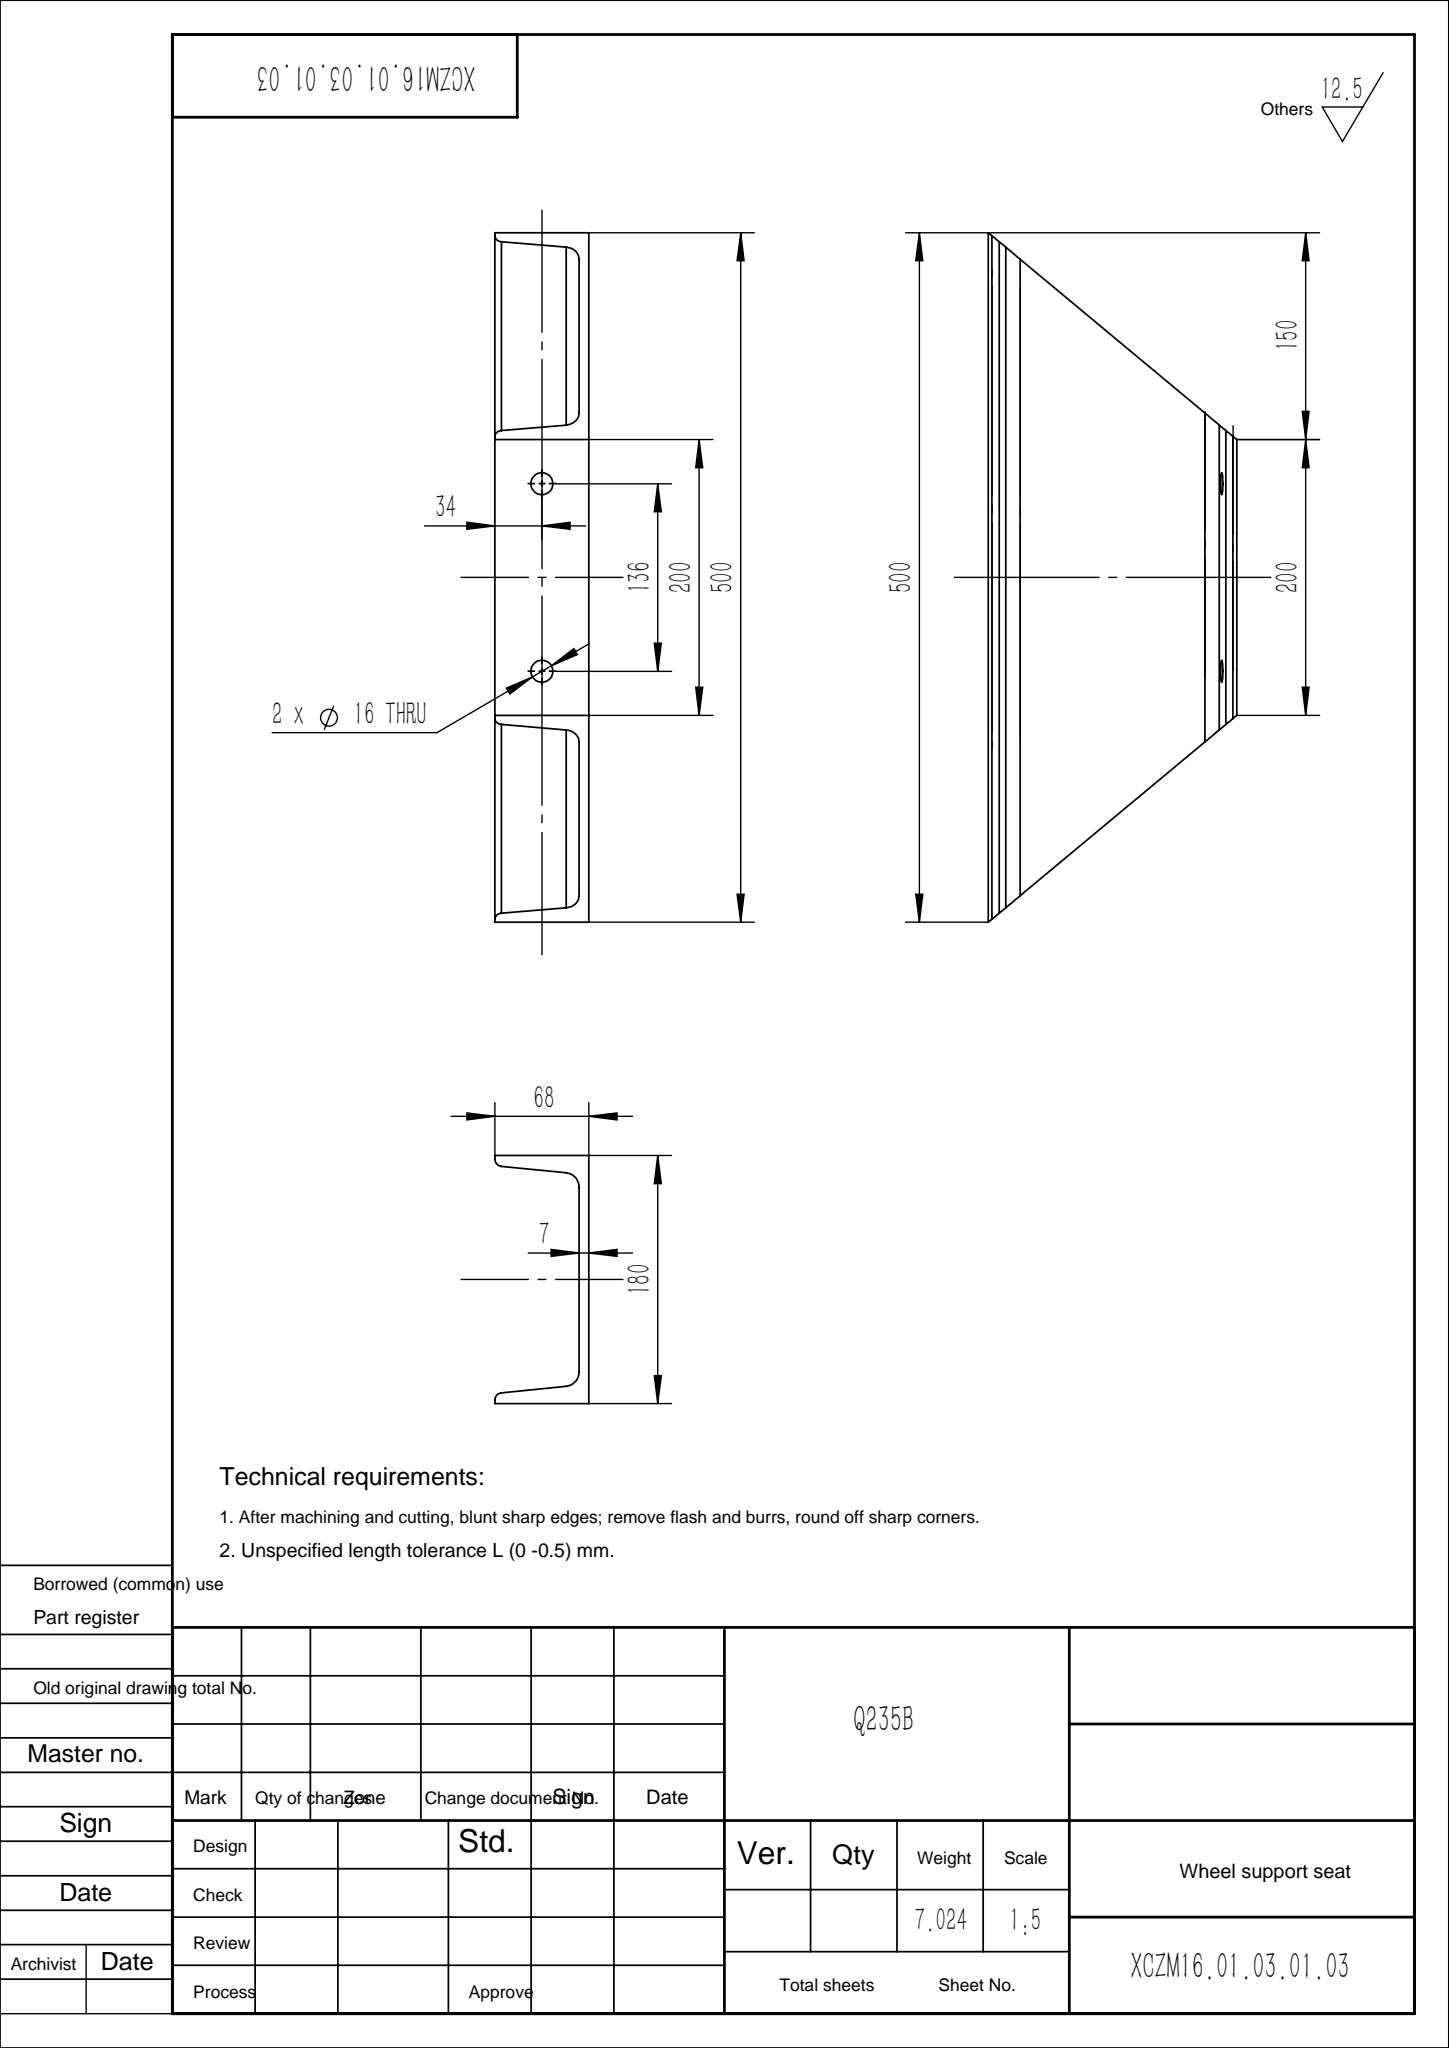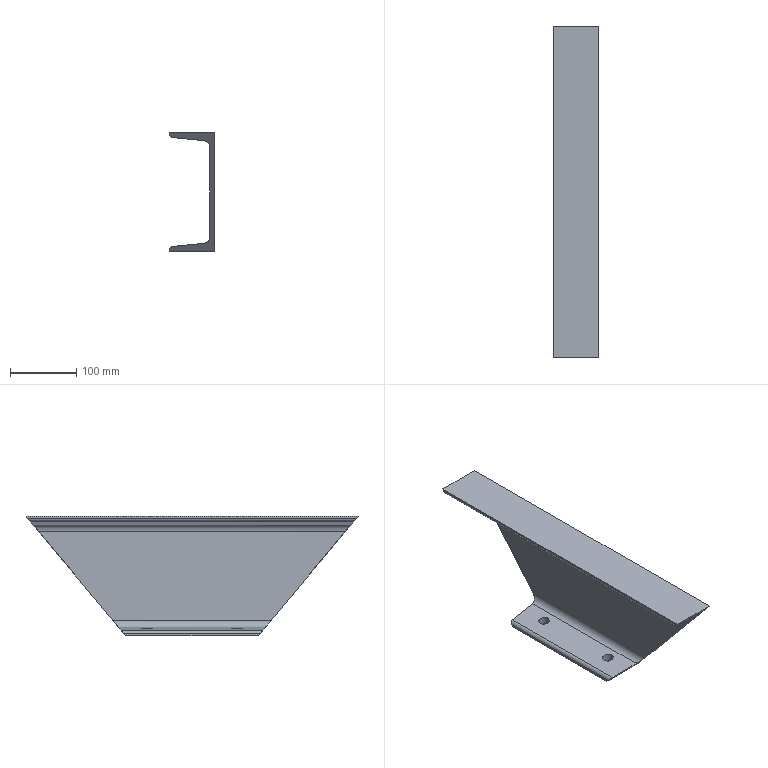Part | SolidWorks | features HoleWzd 1, ICE 1, WeldMemberFeat 1, WeldmentFeature 1 | 1 solid | 18 faces | box 68 x 500 x 180 mm | volume 894795 mm3 | plane 10 | cylinder 8 | commonest cylinder face diameters 16 x4 10.5 x2 21 x2
STEP:
#1=CARTESIAN_POINT('',(-26.,318.,11.65));
#2=VERTEX_POINT('',#1);
#3=CARTESIAN_POINT('',(-42.,318.,10.05));
#4=VERTEX_POINT('',#3);
#5=CARTESIAN_POINT('',(-26.,318.,11.65));
#6=CARTESIAN_POINT('',(-26.,302.,11.65));
#7=CARTESIAN_POINT('',(-42.,302.,10.05));
#8=CARTESIAN_POINT('',(-42.,318.,10.05));
#9=(BOUNDED_CURVE()B_SPLINE_CURVE(3,(#5,#6,#7,#8),.UNSPECIFIED.,.F.,.F.)B_SPLINE_CURVE_WITH_KNOTS((4,4),(3.142,6.283),.UNSPECIFIED.)CURVE()GEOMETRIC_REPRESENTATION_ITEM()RATIONAL_B_SPLINE_CURVE((1.,0.3333,0.3333,1.))REPRESENTATION_ITEM(''));
#10=EDGE_CURVE('',#2,#4,#9,.T.);
#11=ORIENTED_EDGE('',*,*,#10,.F.);
#12=CARTESIAN_POINT('',(-26.,318.,0.));
#13=VERTEX_POINT('',#12);
#14=CARTESIAN_POINT('',(-26.,318.,0.));
#15=DIRECTION('',(0.,0.,-1.));
#16=VECTOR('',#15,1000.);
#17=LINE('',#14,#16);
#18=EDGE_CURVE('',#2,#13,#17,.T.);
#19=ORIENTED_EDGE('',*,*,#18,.T.);
#20=CARTESIAN_POINT('',(-42.,318.,0.));
#21=VERTEX_POINT('',#20);
#22=CARTESIAN_POINT('',(-34.,318.,0.));
#23=DIRECTION('',(0.,0.,-1.));
#24=DIRECTION('',(-1.,0.,0.));
#25=AXIS2_PLACEMENT_3D('',#22,#23,#24);
#26=CIRCLE('',#25,8.);
#27=EDGE_CURVE('',#13,#21,#26,.T.);
#28=ORIENTED_EDGE('',*,*,#27,.T.);
#29=CARTESIAN_POINT('',(-42.,318.,0.));
#30=DIRECTION('',(0.,0.,-1.));
#31=VECTOR('',#30,1000.);
#32=LINE('',#29,#31);
#33=EDGE_CURVE('',#4,#21,#32,.T.);
#34=ORIENTED_EDGE('',*,*,#33,.F.);
#35=EDGE_LOOP('',(#11,#19,#28,#34));
#36=FACE_OUTER_BOUND('',#35,.T.);
#37=CARTESIAN_POINT('',(-34.,318.,0.));
#38=DIRECTION('',(0.,0.,-1.));
#39=DIRECTION('',(-1.,0.,0.));
#40=AXIS2_PLACEMENT_3D('',#37,#38,#39);
#41=CYLINDRICAL_SURFACE('',#40,8.);
#42=ADVANCED_FACE('',(#36),#41,.F.);
#43=CARTESIAN_POINT('',(-26.,182.,11.65));
#44=VERTEX_POINT('',#43);
#45=CARTESIAN_POINT('',(-42.,182.,10.05));
#46=VERTEX_POINT('',#45);
#47=CARTESIAN_POINT('',(-26.,182.,11.65));
#48=CARTESIAN_POINT('',(-26.,166.,11.65));
#49=CARTESIAN_POINT('',(-42.,166.,10.05));
#50=CARTESIAN_POINT('',(-42.,182.,10.05));
#51=(BOUNDED_CURVE()B_SPLINE_CURVE(3,(#47,#48,#49,#50),.UNSPECIFIED.,.F.,.F.)B_SPLINE_CURVE_WITH_KNOTS((4,4),(3.142,6.283),.UNSPECIFIED.)CURVE()GEOMETRIC_REPRESENTATION_ITEM()RATIONAL_B_SPLINE_CURVE((1.,0.3333,0.3333,1.))REPRESENTATION_ITEM(''));
#52=EDGE_CURVE('',#44,#46,#51,.T.);
#53=ORIENTED_EDGE('',*,*,#52,.F.);
#54=CARTESIAN_POINT('',(-26.,182.,0.));
#55=VERTEX_POINT('',#54);
#56=CARTESIAN_POINT('',(-26.,182.,0.));
#57=DIRECTION('',(0.,0.,-1.));
#58=VECTOR('',#57,1000.);
#59=LINE('',#56,#58);
#60=EDGE_CURVE('',#44,#55,#59,.T.);
#61=ORIENTED_EDGE('',*,*,#60,.T.);
#62=CARTESIAN_POINT('',(-42.,182.,0.));
#63=VERTEX_POINT('',#62);
#64=CARTESIAN_POINT('',(-34.,182.,0.));
#65=DIRECTION('',(0.,0.,-1.));
#66=DIRECTION('',(-1.,0.,0.));
#67=AXIS2_PLACEMENT_3D('',#64,#65,#66);
#68=CIRCLE('',#67,8.);
#69=EDGE_CURVE('',#55,#63,#68,.T.);
#70=ORIENTED_EDGE('',*,*,#69,.T.);
#71=CARTESIAN_POINT('',(-42.,182.,0.));
#72=DIRECTION('',(0.,0.,-1.));
#73=VECTOR('',#72,1000.);
#74=LINE('',#71,#73);
#75=EDGE_CURVE('',#46,#63,#74,.T.);
#76=ORIENTED_EDGE('',*,*,#75,.F.);
#77=EDGE_LOOP('',(#53,#61,#70,#76));
#78=FACE_OUTER_BOUND('',#77,.T.);
#79=CARTESIAN_POINT('',(-34.,182.,0.));
#80=DIRECTION('',(0.,0.,-1.));
#81=DIRECTION('',(-1.,0.,0.));
#82=AXIS2_PLACEMENT_3D('',#79,#80,#81);
#83=CYLINDRICAL_SURFACE('',#82,8.);
#84=ADVANCED_FACE('',(#78),#83,.F.);
#85=CARTESIAN_POINT('',(-63.272,493.398,172.077));
#86=VERTEX_POINT('',#85);
#87=CARTESIAN_POINT('',(-68.,497.751,177.301));
#88=VERTEX_POINT('',#87);
#89=CARTESIAN_POINT('',(-63.272,493.398,172.077));
#90=CARTESIAN_POINT('',(-66.096,493.633,172.36));
#91=CARTESIAN_POINT('',(-68.,495.386,174.464));
#92=CARTESIAN_POINT('',(-68.,497.751,177.301));
#93=(BOUNDED_CURVE()B_SPLINE_CURVE(3,(#89,#90,#91,#92),.UNSPECIFIED.,.F.,.F.)B_SPLINE_CURVE_WITH_KNOTS((4,4),(0.09967,1.571),.UNSPECIFIED.)CURVE()GEOMETRIC_REPRESENTATION_ITEM()RATIONAL_B_SPLINE_CURVE((1.,0.8276,0.8276,1.))REPRESENTATION_ITEM(''));
#94=EDGE_CURVE('',#86,#88,#93,.T.);
#95=ORIENTED_EDGE('',*,*,#94,.F.);
#96=CARTESIAN_POINT('',(-63.272,6.602,172.077));
#97=VERTEX_POINT('',#96);
#98=CARTESIAN_POINT('',(-63.272,500.,172.077));
#99=DIRECTION('',(0.,-1.,0.));
#100=VECTOR('',#99,1000.);
#101=LINE('',#98,#100);
#102=EDGE_CURVE('',#86,#97,#101,.T.);
#103=ORIENTED_EDGE('',*,*,#102,.T.);
#104=CARTESIAN_POINT('',(-68.,2.249,177.301));
#105=VERTEX_POINT('',#104);
#106=CARTESIAN_POINT('',(-68.,2.249,177.301));
#107=CARTESIAN_POINT('',(-68.,4.614,174.464));
#108=CARTESIAN_POINT('',(-66.096,6.367,172.36));
#109=CARTESIAN_POINT('',(-63.272,6.602,172.077));
#110=(BOUNDED_CURVE()B_SPLINE_CURVE(3,(#106,#107,#108,#109),.UNSPECIFIED.,.F.,.F.)B_SPLINE_CURVE_WITH_KNOTS((4,4),(1.571,3.042),.UNSPECIFIED.)CURVE()GEOMETRIC_REPRESENTATION_ITEM()RATIONAL_B_SPLINE_CURVE((1.,0.8276,0.8276,1.))REPRESENTATION_ITEM(''));
#111=EDGE_CURVE('',#105,#97,#110,.T.);
#112=ORIENTED_EDGE('',*,*,#111,.F.);
#113=CARTESIAN_POINT('',(-68.,500.,177.301));
#114=DIRECTION('',(0.,-1.,0.));
#115=VECTOR('',#114,1000.);
#116=LINE('',#113,#115);
#117=EDGE_CURVE('',#88,#105,#116,.T.);
#118=ORIENTED_EDGE('',*,*,#117,.F.);
#119=EDGE_LOOP('',(#95,#103,#112,#118));
#120=FACE_OUTER_BOUND('',#119,.T.);
#121=CARTESIAN_POINT('',(-62.75,500.,177.301));
#122=DIRECTION('',(0.,-1.,0.));
#123=DIRECTION('',(0.,0.,-1.));
#124=AXIS2_PLACEMENT_3D('',#121,#122,#123);
#125=CYLINDRICAL_SURFACE('',#124,5.25);
#126=ADVANCED_FACE('',(#120),#125,.T.);
#127=CARTESIAN_POINT('',(-68.,500.,180.));
#128=VERTEX_POINT('',#127);
#129=CARTESIAN_POINT('',(-68.,500.,180.));
#130=DIRECTION('',(0.,0.6402,0.7682));
#131=VECTOR('',#130,1000.);
#132=LINE('',#129,#131);
#133=EDGE_CURVE('',#88,#128,#132,.T.);
#134=ORIENTED_EDGE('',*,*,#133,.F.);
#135=ORIENTED_EDGE('',*,*,#117,.T.);
#136=CARTESIAN_POINT('',(-68.,0.,180.));
#137=VERTEX_POINT('',#136);
#138=CARTESIAN_POINT('',(-68.,0.,180.));
#139=DIRECTION('',(0.,0.6402,-0.7682));
#140=VECTOR('',#139,1000.);
#141=LINE('',#138,#140);
#142=EDGE_CURVE('',#137,#105,#141,.T.);
#143=ORIENTED_EDGE('',*,*,#142,.F.);
#144=CARTESIAN_POINT('',(-68.,500.,180.));
#145=DIRECTION('',(0.,-1.,0.));
#146=VECTOR('',#145,1000.);
#147=LINE('',#144,#146);
#148=EDGE_CURVE('',#128,#137,#147,.T.);
#149=ORIENTED_EDGE('',*,*,#148,.F.);
#150=EDGE_LOOP('',(#134,#135,#143,#149));
#151=FACE_OUTER_BOUND('',#150,.T.);
#152=CARTESIAN_POINT('',(-68.,500.,180.));
#153=DIRECTION('',(1.,0.,0.));
#154=DIRECTION('',(0.,0.,-1.));
#155=AXIS2_PLACEMENT_3D('',#152,#153,#154);
#156=PLANE('',#155);
#157=ADVANCED_FACE('',(#151),#156,.F.);
#158=CARTESIAN_POINT('',(0.,350.,0.));
#159=VERTEX_POINT('',#158);
#160=CARTESIAN_POINT('',(0.,500.,180.));
#161=VERTEX_POINT('',#160);
#162=CARTESIAN_POINT('',(0.,500.,180.));
#163=DIRECTION('',(0.,0.6402,0.7682));
#164=VECTOR('',#163,1000.);
#165=LINE('',#162,#164);
#166=EDGE_CURVE('',#159,#161,#165,.T.);
#167=ORIENTED_EDGE('',*,*,#166,.T.);
#168=CARTESIAN_POINT('',(0.,0.,180.));
#169=VERTEX_POINT('',#168);
#170=CARTESIAN_POINT('',(0.,500.,180.));
#171=DIRECTION('',(0.,-1.,0.));
#172=VECTOR('',#171,1000.);
#173=LINE('',#170,#172);
#174=EDGE_CURVE('',#161,#169,#173,.T.);
#175=ORIENTED_EDGE('',*,*,#174,.T.);
#176=CARTESIAN_POINT('',(0.,150.,0.));
#177=VERTEX_POINT('',#176);
#178=CARTESIAN_POINT('',(0.,0.,180.));
#179=DIRECTION('',(0.,0.6402,-0.7682));
#180=VECTOR('',#179,1000.);
#181=LINE('',#178,#180);
#182=EDGE_CURVE('',#169,#177,#181,.T.);
#183=ORIENTED_EDGE('',*,*,#182,.T.);
#184=CARTESIAN_POINT('',(0.,500.,0.));
#185=DIRECTION('',(0.,-1.,0.));
#186=VECTOR('',#185,1000.);
#187=LINE('',#184,#186);
#188=EDGE_CURVE('',#159,#177,#187,.T.);
#189=ORIENTED_EDGE('',*,*,#188,.F.);
#190=EDGE_LOOP('',(#167,#175,#183,#189));
#191=FACE_OUTER_BOUND('',#190,.T.);
#192=CARTESIAN_POINT('',(0.,500.,180.));
#193=DIRECTION('',(-1.,0.,0.));
#194=DIRECTION('',(0.,0.,1.));
#195=AXIS2_PLACEMENT_3D('',#192,#193,#194);
#196=PLANE('',#195);
#197=ADVANCED_FACE('',(#191),#196,.F.);
#198=CARTESIAN_POINT('',(-34.,318.,0.));
#199=DIRECTION('',(0.,0.,-1.));
#200=DIRECTION('',(-1.,0.,0.));
#201=AXIS2_PLACEMENT_3D('',#198,#199,#200);
#202=CIRCLE('',#201,8.);
#203=EDGE_CURVE('',#21,#13,#202,.T.);
#204=ORIENTED_EDGE('',*,*,#203,.F.);
#205=ORIENTED_EDGE('',*,*,#27,.F.);
#206=EDGE_LOOP('',(#204,#205));
#207=FACE_BOUND('',#206,.T.);
#208=CARTESIAN_POINT('',(-34.,182.,0.));
#209=DIRECTION('',(0.,0.,-1.));
#210=DIRECTION('',(-1.,0.,0.));
#211=AXIS2_PLACEMENT_3D('',#208,#209,#210);
#212=CIRCLE('',#211,8.);
#213=EDGE_CURVE('',#63,#55,#212,.T.);
#214=ORIENTED_EDGE('',*,*,#213,.F.);
#215=ORIENTED_EDGE('',*,*,#69,.F.);
#216=EDGE_LOOP('',(#214,#215));
#217=FACE_BOUND('',#216,.T.);
#218=CARTESIAN_POINT('',(-68.,350.,0.));
#219=VERTEX_POINT('',#218);
#220=CARTESIAN_POINT('',(-68.,350.,0.));
#221=DIRECTION('',(1.,0.,0.));
#222=VECTOR('',#221,1000.);
#223=LINE('',#220,#222);
#224=EDGE_CURVE('',#219,#159,#223,.T.);
#225=ORIENTED_EDGE('',*,*,#224,.T.);
#226=ORIENTED_EDGE('',*,*,#188,.T.);
#227=CARTESIAN_POINT('',(-68.,150.,0.));
#228=VERTEX_POINT('',#227);
#229=CARTESIAN_POINT('',(-68.,150.,0.));
#230=DIRECTION('',(1.,0.,0.));
#231=VECTOR('',#230,1000.);
#232=LINE('',#229,#231);
#233=EDGE_CURVE('',#228,#177,#232,.T.);
#234=ORIENTED_EDGE('',*,*,#233,.F.);
#235=CARTESIAN_POINT('',(-68.,500.,0.));
#236=DIRECTION('',(0.,-1.,0.));
#237=VECTOR('',#236,1000.);
#238=LINE('',#235,#237);
#239=EDGE_CURVE('',#219,#228,#238,.T.);
#240=ORIENTED_EDGE('',*,*,#239,.F.);
#241=EDGE_LOOP('',(#225,#226,#234,#240));
#242=FACE_OUTER_BOUND('',#241,.T.);
#243=CARTESIAN_POINT('',(-68.,500.,0.));
#244=DIRECTION('',(0.,0.,1.));
#245=DIRECTION('',(1.,0.,0.));
#246=AXIS2_PLACEMENT_3D('',#243,#244,#245);
#247=PLANE('',#246);
#248=ADVANCED_FACE('',(#207,#217,#242),#247,.F.);
#249=CARTESIAN_POINT('',(-68.,352.249,2.699));
#250=VERTEX_POINT('',#249);
#251=CARTESIAN_POINT('',(-68.,500.,180.));
#252=DIRECTION('',(0.,0.6402,0.7682));
#253=VECTOR('',#252,1000.);
#254=LINE('',#251,#253);
#255=EDGE_CURVE('',#219,#250,#254,.T.);
#256=ORIENTED_EDGE('',*,*,#255,.F.);
#257=ORIENTED_EDGE('',*,*,#239,.T.);
#258=CARTESIAN_POINT('',(-68.,147.751,2.699));
#259=VERTEX_POINT('',#258);
#260=CARTESIAN_POINT('',(-68.,0.,180.));
#261=DIRECTION('',(0.,0.6402,-0.7682));
#262=VECTOR('',#261,1000.);
#263=LINE('',#260,#262);
#264=EDGE_CURVE('',#259,#228,#263,.T.);
#265=ORIENTED_EDGE('',*,*,#264,.F.);
#266=CARTESIAN_POINT('',(-68.,500.,2.699));
#267=DIRECTION('',(0.,-1.,0.));
#268=VECTOR('',#267,1000.);
#269=LINE('',#266,#268);
#270=EDGE_CURVE('',#250,#259,#269,.T.);
#271=ORIENTED_EDGE('',*,*,#270,.F.);
#272=EDGE_LOOP('',(#256,#257,#265,#271));
#273=FACE_OUTER_BOUND('',#272,.T.);
#274=CARTESIAN_POINT('',(-68.,500.,0.));
#275=DIRECTION('',(1.,0.,0.));
#276=DIRECTION('',(0.,0.,-1.));
#277=AXIS2_PLACEMENT_3D('',#274,#275,#276);
#278=PLANE('',#277);
#279=ADVANCED_FACE('',(#273),#278,.F.);
#280=CARTESIAN_POINT('',(-63.272,356.602,7.923));
#281=VERTEX_POINT('',#280);
#282=CARTESIAN_POINT('',(-68.,352.249,2.699));
#283=CARTESIAN_POINT('',(-68.,354.614,5.536));
#284=CARTESIAN_POINT('',(-66.096,356.367,7.64));
#285=CARTESIAN_POINT('',(-63.272,356.602,7.923));
#286=(BOUNDED_CURVE()B_SPLINE_CURVE(3,(#282,#283,#284,#285),.UNSPECIFIED.,.F.,.F.)B_SPLINE_CURVE_WITH_KNOTS((4,4),(1.571,3.042),.UNSPECIFIED.)CURVE()GEOMETRIC_REPRESENTATION_ITEM()RATIONAL_B_SPLINE_CURVE((1.,0.8276,0.8276,1.))REPRESENTATION_ITEM(''));
#287=EDGE_CURVE('',#250,#281,#286,.T.);
#288=ORIENTED_EDGE('',*,*,#287,.F.);
#289=ORIENTED_EDGE('',*,*,#270,.T.);
#290=CARTESIAN_POINT('',(-63.272,143.398,7.923));
#291=VERTEX_POINT('',#290);
#292=CARTESIAN_POINT('',(-63.272,143.398,7.923));
#293=CARTESIAN_POINT('',(-66.096,143.633,7.64));
#294=CARTESIAN_POINT('',(-68.,145.386,5.536));
#295=CARTESIAN_POINT('',(-68.,147.751,2.699));
#296=(BOUNDED_CURVE()B_SPLINE_CURVE(3,(#292,#293,#294,#295),.UNSPECIFIED.,.F.,.F.)B_SPLINE_CURVE_WITH_KNOTS((4,4),(0.09967,1.571),.UNSPECIFIED.)CURVE()GEOMETRIC_REPRESENTATION_ITEM()RATIONAL_B_SPLINE_CURVE((1.,0.8276,0.8276,1.))REPRESENTATION_ITEM(''));
#297=EDGE_CURVE('',#291,#259,#296,.T.);
#298=ORIENTED_EDGE('',*,*,#297,.F.);
#299=CARTESIAN_POINT('',(-63.272,500.,7.923));
#300=DIRECTION('',(0.,-1.,0.));
#301=VECTOR('',#300,1000.);
#302=LINE('',#299,#301);
#303=EDGE_CURVE('',#281,#291,#302,.T.);
#304=ORIENTED_EDGE('',*,*,#303,.F.);
#305=EDGE_LOOP('',(#288,#289,#298,#304));
#306=FACE_OUTER_BOUND('',#305,.T.);
#307=CARTESIAN_POINT('',(-62.75,500.,2.699));
#308=DIRECTION('',(0.,-1.,0.));
#309=DIRECTION('',(0.,0.,-1.));
#310=AXIS2_PLACEMENT_3D('',#307,#308,#309);
#311=CYLINDRICAL_SURFACE('',#310,5.25);
#312=ADVANCED_FACE('',(#306),#311,.T.);
#313=CARTESIAN_POINT('',(-42.,318.,10.05));
#314=CARTESIAN_POINT('',(-42.,334.,10.05));
#315=CARTESIAN_POINT('',(-26.,334.,11.65));
#316=CARTESIAN_POINT('',(-26.,318.,11.65));
#317=(BOUNDED_CURVE()B_SPLINE_CURVE(3,(#313,#314,#315,#316),.UNSPECIFIED.,.F.,.F.)B_SPLINE_CURVE_WITH_KNOTS((4,4),(0.,3.142),.UNSPECIFIED.)CURVE()GEOMETRIC_REPRESENTATION_ITEM()RATIONAL_B_SPLINE_CURVE((1.,0.3333,0.3333,1.))REPRESENTATION_ITEM(''));
#318=EDGE_CURVE('',#4,#2,#317,.T.);
#319=ORIENTED_EDGE('',*,*,#318,.T.);
#320=ORIENTED_EDGE('',*,*,#10,.T.);
#321=EDGE_LOOP('',(#319,#320));
#322=FACE_BOUND('',#321,.T.);
#323=CARTESIAN_POINT('',(-42.,182.,10.05));
#324=CARTESIAN_POINT('',(-42.,198.,10.05));
#325=CARTESIAN_POINT('',(-26.,198.,11.65));
#326=CARTESIAN_POINT('',(-26.,182.,11.65));
#327=(BOUNDED_CURVE()B_SPLINE_CURVE(3,(#323,#324,#325,#326),.UNSPECIFIED.,.F.,.F.)B_SPLINE_CURVE_WITH_KNOTS((4,4),(0.,3.142),.UNSPECIFIED.)CURVE()GEOMETRIC_REPRESENTATION_ITEM()RATIONAL_B_SPLINE_CURVE((1.,0.3333,0.3333,1.))REPRESENTATION_ITEM(''));
#328=EDGE_CURVE('',#46,#44,#327,.T.);
#329=ORIENTED_EDGE('',*,*,#328,.T.);
#330=ORIENTED_EDGE('',*,*,#52,.T.);
#331=EDGE_LOOP('',(#329,#330));
#332=FACE_BOUND('',#331,.T.);
#333=CARTESIAN_POINT('',(-16.455,360.504,12.604));
#334=VERTEX_POINT('',#333);
#335=CARTESIAN_POINT('',(-5.024,361.456,13.748));
#336=DIRECTION('',(0.9916,0.08264,0.09916));
#337=VECTOR('',#336,1000.);
#338=LINE('',#335,#337);
#339=EDGE_CURVE('',#281,#334,#338,.T.);
#340=ORIENTED_EDGE('',*,*,#339,.F.);
#341=ORIENTED_EDGE('',*,*,#303,.T.);
#342=CARTESIAN_POINT('',(-16.455,139.496,12.604));
#343=VERTEX_POINT('',#342);
#344=CARTESIAN_POINT('',(-45.997,141.958,9.65));
#345=DIRECTION('',(-0.9916,0.08264,-0.09916));
#346=VECTOR('',#345,1000.);
#347=LINE('',#344,#346);
#348=EDGE_CURVE('',#343,#291,#347,.T.);
#349=ORIENTED_EDGE('',*,*,#348,.F.);
#350=CARTESIAN_POINT('',(-16.455,500.,12.604));
#351=DIRECTION('',(0.,-1.,0.));
#352=VECTOR('',#351,1000.);
#353=LINE('',#350,#352);
#354=EDGE_CURVE('',#334,#343,#353,.T.);
#355=ORIENTED_EDGE('',*,*,#354,.F.);
#356=EDGE_LOOP('',(#340,#341,#349,#355));
#357=FACE_OUTER_BOUND('',#356,.T.);
#358=CARTESIAN_POINT('',(-16.455,500.,12.604));
#359=DIRECTION('',(0.0995,0.,-0.995));
#360=DIRECTION('',(-0.995,0.,-0.0995));
#361=AXIS2_PLACEMENT_3D('',#358,#359,#360);
#362=PLANE('',#361);
#363=ADVANCED_FACE('',(#322,#332,#357),#362,.F.);
#364=CARTESIAN_POINT('',(-7.,369.21,23.052));
#365=VERTEX_POINT('',#364);
#366=CARTESIAN_POINT('',(-16.455,360.504,12.604));
#367=CARTESIAN_POINT('',(-10.808,360.974,13.169));
#368=CARTESIAN_POINT('',(-7.,364.481,17.377));
#369=CARTESIAN_POINT('',(-7.,369.21,23.052));
#370=(BOUNDED_CURVE()B_SPLINE_CURVE(3,(#366,#367,#368,#369),.UNSPECIFIED.,.F.,.F.)B_SPLINE_CURVE_WITH_KNOTS((4,4),(0.09967,1.571),.UNSPECIFIED.)CURVE()GEOMETRIC_REPRESENTATION_ITEM()RATIONAL_B_SPLINE_CURVE((1.,0.8276,0.8276,1.))REPRESENTATION_ITEM(''));
#371=EDGE_CURVE('',#334,#365,#370,.T.);
#372=ORIENTED_EDGE('',*,*,#371,.F.);
#373=ORIENTED_EDGE('',*,*,#354,.T.);
#374=CARTESIAN_POINT('',(-7.,130.79,23.052));
#375=VERTEX_POINT('',#374);
#376=CARTESIAN_POINT('',(-7.,130.79,23.052));
#377=CARTESIAN_POINT('',(-7.,135.519,17.377));
#378=CARTESIAN_POINT('',(-10.808,139.026,13.169));
#379=CARTESIAN_POINT('',(-16.455,139.496,12.604));
#380=(BOUNDED_CURVE()B_SPLINE_CURVE(3,(#376,#377,#378,#379),.UNSPECIFIED.,.F.,.T.)B_SPLINE_CURVE_WITH_KNOTS((4,4),(1.571,3.042),.UNSPECIFIED.)CURVE()GEOMETRIC_REPRESENTATION_ITEM()RATIONAL_B_SPLINE_CURVE((1.,0.8276,0.8276,1.))REPRESENTATION_ITEM(''));
#381=EDGE_CURVE('',#375,#343,#380,.T.);
#382=ORIENTED_EDGE('',*,*,#381,.F.);
#383=CARTESIAN_POINT('',(-7.,500.,23.052));
#384=DIRECTION('',(0.,-1.,0.));
#385=VECTOR('',#384,1000.);
#386=LINE('',#383,#385);
#387=EDGE_CURVE('',#365,#375,#386,.T.);
#388=ORIENTED_EDGE('',*,*,#387,.F.);
#389=EDGE_LOOP('',(#372,#373,#382,#388));
#390=FACE_OUTER_BOUND('',#389,.T.);
#391=CARTESIAN_POINT('',(-17.5,500.,23.052));
#392=DIRECTION('',(0.,-1.,0.));
#393=DIRECTION('',(0.,0.,-1.));
#394=AXIS2_PLACEMENT_3D('',#391,#392,#393);
#395=CYLINDRICAL_SURFACE('',#394,10.5);
#396=ADVANCED_FACE('',(#390),#395,.F.);
#397=CARTESIAN_POINT('',(-7.,480.79,156.948));
#398=VERTEX_POINT('',#397);
#399=CARTESIAN_POINT('',(-7.,488.663,166.395));
#400=DIRECTION('',(0.,0.6402,0.7682));
#401=VECTOR('',#400,1000.);
#402=LINE('',#399,#401);
#403=EDGE_CURVE('',#365,#398,#402,.T.);
#404=ORIENTED_EDGE('',*,*,#403,.F.);
#405=ORIENTED_EDGE('',*,*,#387,.T.);
#406=CARTESIAN_POINT('',(-7.,19.21,156.948));
#407=VERTEX_POINT('',#406);
#408=CARTESIAN_POINT('',(-7.,216.255,-79.506));
#409=DIRECTION('',(0.,0.6402,-0.7682));
#410=VECTOR('',#409,1000.);
#411=LINE('',#408,#410);
#412=EDGE_CURVE('',#407,#375,#411,.T.);
#413=ORIENTED_EDGE('',*,*,#412,.F.);
#414=CARTESIAN_POINT('',(-7.,500.,156.948));
#415=DIRECTION('',(0.,-1.,0.));
#416=VECTOR('',#415,1000.);
#417=LINE('',#414,#416);
#418=EDGE_CURVE('',#398,#407,#417,.T.);
#419=ORIENTED_EDGE('',*,*,#418,.F.);
#420=EDGE_LOOP('',(#404,#405,#413,#419));
#421=FACE_OUTER_BOUND('',#420,.T.);
#422=CARTESIAN_POINT('',(-7.,500.,156.948));
#423=DIRECTION('',(1.,0.,0.));
#424=DIRECTION('',(0.,0.,-1.));
#425=AXIS2_PLACEMENT_3D('',#422,#423,#424);
#426=PLANE('',#425);
#427=ADVANCED_FACE('',(#421),#426,.F.);
#428=CARTESIAN_POINT('',(-16.455,489.496,167.396));
#429=VERTEX_POINT('',#428);
#430=CARTESIAN_POINT('',(-7.,480.79,156.948));
#431=CARTESIAN_POINT('',(-7.,485.519,162.623));
#432=CARTESIAN_POINT('',(-10.808,489.026,166.831));
#433=CARTESIAN_POINT('',(-16.455,489.496,167.396));
#434=(BOUNDED_CURVE()B_SPLINE_CURVE(3,(#430,#431,#432,#433),.UNSPECIFIED.,.F.,.F.)B_SPLINE_CURVE_WITH_KNOTS((4,4),(1.571,3.042),.UNSPECIFIED.)CURVE()GEOMETRIC_REPRESENTATION_ITEM()RATIONAL_B_SPLINE_CURVE((1.,0.8276,0.8276,1.))REPRESENTATION_ITEM(''));
#435=EDGE_CURVE('',#398,#429,#434,.T.);
#436=ORIENTED_EDGE('',*,*,#435,.F.);
#437=ORIENTED_EDGE('',*,*,#418,.T.);
#438=CARTESIAN_POINT('',(-16.455,10.504,167.396));
#439=VERTEX_POINT('',#438);
#440=CARTESIAN_POINT('',(-16.455,10.504,167.396));
#441=CARTESIAN_POINT('',(-10.808,10.974,166.831));
#442=CARTESIAN_POINT('',(-7.,14.481,162.623));
#443=CARTESIAN_POINT('',(-7.,19.21,156.948));
#444=(BOUNDED_CURVE()B_SPLINE_CURVE(3,(#440,#441,#442,#443),.UNSPECIFIED.,.F.,.F.)B_SPLINE_CURVE_WITH_KNOTS((4,4),(0.09967,1.571),.UNSPECIFIED.)CURVE()GEOMETRIC_REPRESENTATION_ITEM()RATIONAL_B_SPLINE_CURVE((1.,0.8276,0.8276,1.))REPRESENTATION_ITEM(''));
#445=EDGE_CURVE('',#439,#407,#444,.T.);
#446=ORIENTED_EDGE('',*,*,#445,.F.);
#447=CARTESIAN_POINT('',(-16.455,500.,167.396));
#448=DIRECTION('',(0.,-1.,0.));
#449=VECTOR('',#448,1000.);
#450=LINE('',#447,#449);
#451=EDGE_CURVE('',#429,#439,#450,.T.);
#452=ORIENTED_EDGE('',*,*,#451,.F.);
#453=EDGE_LOOP('',(#436,#437,#446,#452));
#454=FACE_OUTER_BOUND('',#453,.T.);
#455=CARTESIAN_POINT('',(-17.5,500.,156.948));
#456=DIRECTION('',(0.,-1.,0.));
#457=DIRECTION('',(0.,0.,-1.));
#458=AXIS2_PLACEMENT_3D('',#455,#456,#457);
#459=CYLINDRICAL_SURFACE('',#458,10.5);
#460=ADVANCED_FACE('',(#454),#459,.F.);
#461=CARTESIAN_POINT('',(-17.316,489.568,167.482));
#462=DIRECTION('',(-0.9916,0.08264,0.09916));
#463=VECTOR('',#462,1000.);
#464=LINE('',#461,#463);
#465=EDGE_CURVE('',#429,#86,#464,.T.);
#466=ORIENTED_EDGE('',*,*,#465,.F.);
#467=ORIENTED_EDGE('',*,*,#451,.T.);
#468=CARTESIAN_POINT('',(23.656,13.846,163.384));
#469=DIRECTION('',(0.9916,0.08264,-0.09916));
#470=VECTOR('',#469,1000.);
#471=LINE('',#468,#470);
#472=EDGE_CURVE('',#97,#439,#471,.T.);
#473=ORIENTED_EDGE('',*,*,#472,.F.);
#474=ORIENTED_EDGE('',*,*,#102,.F.);
#475=EDGE_LOOP('',(#466,#467,#473,#474));
#476=FACE_OUTER_BOUND('',#475,.T.);
#477=CARTESIAN_POINT('',(-16.455,500.,167.396));
#478=DIRECTION('',(0.0995,0.,0.995));
#479=DIRECTION('',(0.995,0.,-0.0995));
#480=AXIS2_PLACEMENT_3D('',#477,#478,#479);
#481=PLANE('',#480);
#482=ADVANCED_FACE('',(#476),#481,.F.);
#483=CARTESIAN_POINT('',(-68.,0.,180.));
#484=DIRECTION('',(1.,0.,0.));
#485=VECTOR('',#484,1000.);
#486=LINE('',#483,#485);
#487=EDGE_CURVE('',#137,#169,#486,.T.);
#488=ORIENTED_EDGE('',*,*,#487,.T.);
#489=ORIENTED_EDGE('',*,*,#174,.F.);
#490=CARTESIAN_POINT('',(-68.,500.,180.));
#491=DIRECTION('',(1.,0.,0.));
#492=VECTOR('',#491,1000.);
#493=LINE('',#490,#492);
#494=EDGE_CURVE('',#128,#161,#493,.T.);
#495=ORIENTED_EDGE('',*,*,#494,.F.);
#496=ORIENTED_EDGE('',*,*,#148,.T.);
#497=EDGE_LOOP('',(#488,#489,#495,#496));
#498=FACE_OUTER_BOUND('',#497,.T.);
#499=CARTESIAN_POINT('',(-68.,500.,180.));
#500=DIRECTION('',(0.,0.,-1.));
#501=DIRECTION('',(-1.,0.,0.));
#502=AXIS2_PLACEMENT_3D('',#499,#500,#501);
#503=PLANE('',#502);
#504=ADVANCED_FACE('',(#498),#503,.F.);
#505=ORIENTED_EDGE('',*,*,#111,.T.);
#506=ORIENTED_EDGE('',*,*,#472,.T.);
#507=ORIENTED_EDGE('',*,*,#445,.T.);
#508=ORIENTED_EDGE('',*,*,#412,.T.);
#509=ORIENTED_EDGE('',*,*,#381,.T.);
#510=ORIENTED_EDGE('',*,*,#348,.T.);
#511=ORIENTED_EDGE('',*,*,#297,.T.);
#512=ORIENTED_EDGE('',*,*,#264,.T.);
#513=ORIENTED_EDGE('',*,*,#233,.T.);
#514=ORIENTED_EDGE('',*,*,#182,.F.);
#515=ORIENTED_EDGE('',*,*,#487,.F.);
#516=ORIENTED_EDGE('',*,*,#142,.T.);
#517=EDGE_LOOP('',(#505,#506,#507,#508,#509,#510,#511,#512,#513,#514,#515,#516));
#518=FACE_OUTER_BOUND('',#517,.T.);
#519=CARTESIAN_POINT('',(-68.,0.,180.));
#520=DIRECTION('',(0.,-0.7682,-0.6402));
#521=DIRECTION('',(0.,0.6402,-0.7682));
#522=AXIS2_PLACEMENT_3D('',#519,#520,#521);
#523=PLANE('',#522);
#524=ADVANCED_FACE('',(#518),#523,.T.);
#525=ORIENTED_EDGE('',*,*,#94,.T.);
#526=ORIENTED_EDGE('',*,*,#133,.T.);
#527=ORIENTED_EDGE('',*,*,#494,.T.);
#528=ORIENTED_EDGE('',*,*,#166,.F.);
#529=ORIENTED_EDGE('',*,*,#224,.F.);
#530=ORIENTED_EDGE('',*,*,#255,.T.);
#531=ORIENTED_EDGE('',*,*,#287,.T.);
#532=ORIENTED_EDGE('',*,*,#339,.T.);
#533=ORIENTED_EDGE('',*,*,#371,.T.);
#534=ORIENTED_EDGE('',*,*,#403,.T.);
#535=ORIENTED_EDGE('',*,*,#435,.T.);
#536=ORIENTED_EDGE('',*,*,#465,.T.);
#537=EDGE_LOOP('',(#525,#526,#527,#528,#529,#530,#531,#532,#533,#534,#535,#536));
#538=FACE_OUTER_BOUND('',#537,.T.);
#539=CARTESIAN_POINT('',(-68.,500.,180.));
#540=DIRECTION('',(0.,0.7682,-0.6402));
#541=DIRECTION('',(0.,0.6402,0.7682));
#542=AXIS2_PLACEMENT_3D('',#539,#540,#541);
#543=PLANE('',#542);
#544=ADVANCED_FACE('',(#538),#543,.T.);
#545=ORIENTED_EDGE('',*,*,#60,.F.);
#546=ORIENTED_EDGE('',*,*,#328,.F.);
#547=ORIENTED_EDGE('',*,*,#75,.T.);
#548=ORIENTED_EDGE('',*,*,#213,.T.);
#549=EDGE_LOOP('',(#545,#546,#547,#548));
#550=FACE_OUTER_BOUND('',#549,.T.);
#551=CARTESIAN_POINT('',(-34.,182.,0.));
#552=DIRECTION('',(0.,0.,-1.));
#553=DIRECTION('',(-1.,0.,0.));
#554=AXIS2_PLACEMENT_3D('',#551,#552,#553);
#555=CYLINDRICAL_SURFACE('',#554,8.);
#556=ADVANCED_FACE('',(#550),#555,.F.);
#557=ORIENTED_EDGE('',*,*,#18,.F.);
#558=ORIENTED_EDGE('',*,*,#318,.F.);
#559=ORIENTED_EDGE('',*,*,#33,.T.);
#560=ORIENTED_EDGE('',*,*,#203,.T.);
#561=EDGE_LOOP('',(#557,#558,#559,#560));
#562=FACE_OUTER_BOUND('',#561,.T.);
#563=CARTESIAN_POINT('',(-34.,318.,0.));
#564=DIRECTION('',(0.,0.,-1.));
#565=DIRECTION('',(-1.,0.,0.));
#566=AXIS2_PLACEMENT_3D('',#563,#564,#565);
#567=CYLINDRICAL_SURFACE('',#566,8.);
#568=ADVANCED_FACE('',(#562),#567,.F.);
#569=CLOSED_SHELL('',(#42,#84,#126,#157,#197,#248,#279,#312,#363,#396,#427,#460,#482,#504,#524,#544,#556,#568));
#570=MANIFOLD_SOLID_BREP('',#569);
#571=CARTESIAN_POINT('',(0.,0.,0.));
#572=DIRECTION('',(0.,0.,1.));
#573=DIRECTION('',(1.,0.,0.));
#574=AXIS2_PLACEMENT_3D('',#571,#572,#573);
#575=(LENGTH_UNIT()NAMED_UNIT(*)SI_UNIT(.MILLI.,.METRE.));
#576=UNCERTAINTY_MEASURE_WITH_UNIT(LENGTH_MEASURE(0.00001),#575,'','');
#577=(NAMED_UNIT(*)PLANE_ANGLE_UNIT()SI_UNIT($,.RADIAN.));
#578=(NAMED_UNIT(*)SI_UNIT($,.STERADIAN.)SOLID_ANGLE_UNIT());
#579=(GEOMETRIC_REPRESENTATION_CONTEXT(3)GLOBAL_UNCERTAINTY_ASSIGNED_CONTEXT((#576))GLOBAL_UNIT_ASSIGNED_CONTEXT((#575,#577,#578))REPRESENTATION_CONTEXT('',''));
#580=ADVANCED_BREP_SHAPE_REPRESENTATION('',(#570,#574),#579);